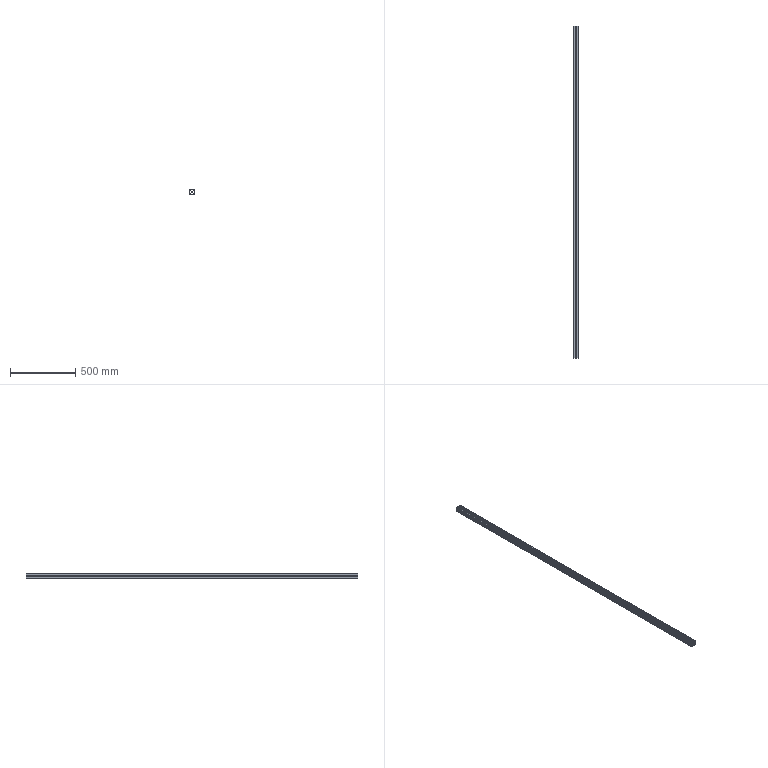Part | SolidWorks | features WeldMemberFeat 1, WeldmentFeature 1 | 1 solid | 104 faces | box 40 x 2550 x 40 mm | volume 1210907 mm3 | plane 94 | cylinder 10 | commonest cylinder face diameters 5 x4 9 x4 6.8 x2